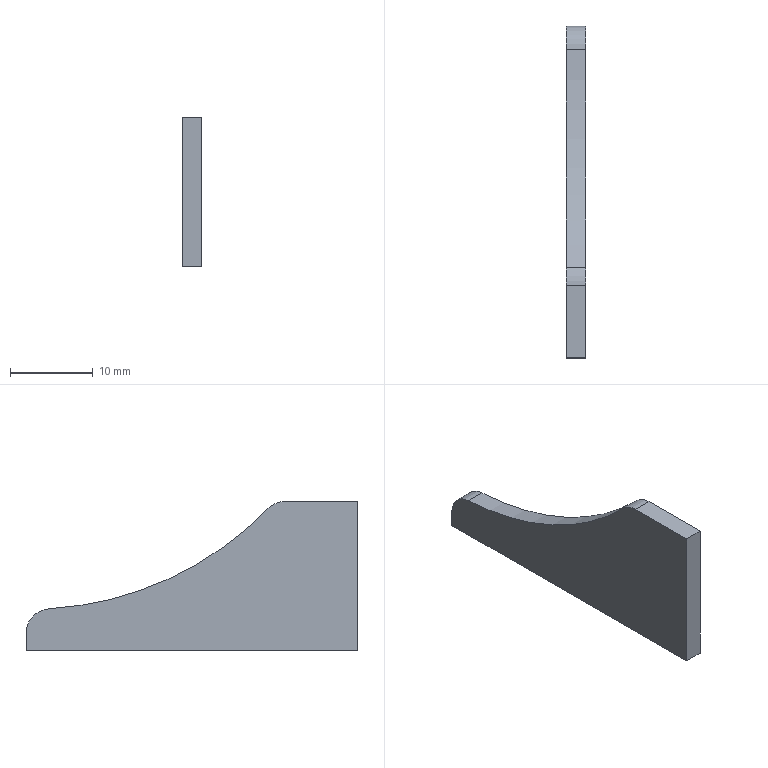Part | SolidWorks | features Fillet 1, FlatPattern 1, SMBaseFlange 1, SheetMetal 1 | 1 solid | 9 faces | box 2.3 x 40 x 18 mm | volume 1026 mm3 | plane 6 | cylinder 3 | commonest cylinder face diameters 6 x2 80 x1
STEP:
#1=CARTESIAN_POINT('',(0.,8.707,18.));
#2=VERTEX_POINT('',#1);
#3=CARTESIAN_POINT('',(0.,0.,18.));
#4=VERTEX_POINT('',#3);
#5=CARTESIAN_POINT('',(0.,10.,18.));
#6=DIRECTION('',(0.,-1.,0.));
#7=VECTOR('',#6,1000.);
#8=LINE('',#5,#7);
#9=EDGE_CURVE('',#2,#4,#8,.T.);
#10=ORIENTED_EDGE('',*,*,#9,.F.);
#11=CARTESIAN_POINT('',(-2.3,8.707,18.));
#12=VERTEX_POINT('',#11);
#13=CARTESIAN_POINT('',(-2.3,8.707,18.));
#14=DIRECTION('',(-1.,0.,0.));
#15=VECTOR('',#14,1000.);
#16=LINE('',#13,#15);
#17=EDGE_CURVE('',#2,#12,#16,.T.);
#18=ORIENTED_EDGE('',*,*,#17,.T.);
#19=CARTESIAN_POINT('',(-2.3,0.,18.));
#20=VERTEX_POINT('',#19);
#21=CARTESIAN_POINT('',(-2.3,10.,18.));
#22=DIRECTION('',(0.,-1.,0.));
#23=VECTOR('',#22,1000.);
#24=LINE('',#21,#23);
#25=EDGE_CURVE('',#12,#20,#24,.T.);
#26=ORIENTED_EDGE('',*,*,#25,.T.);
#27=CARTESIAN_POINT('',(-2.3,0.,18.));
#28=DIRECTION('',(1.,0.,0.));
#29=VECTOR('',#28,1000.);
#30=LINE('',#27,#29);
#31=EDGE_CURVE('',#20,#4,#30,.T.);
#32=ORIENTED_EDGE('',*,*,#31,.T.);
#33=EDGE_LOOP('',(#10,#18,#26,#32));
#34=FACE_OUTER_BOUND('',#33,.T.);
#35=CARTESIAN_POINT('',(-2.3,10.,18.));
#36=DIRECTION('',(0.,0.,1.));
#37=DIRECTION('',(1.,0.,0.));
#38=AXIS2_PLACEMENT_3D('',#35,#36,#37);
#39=PLANE('',#38);
#40=ADVANCED_FACE('',(#34),#39,.T.);
#41=CARTESIAN_POINT('',(-2.3,37.175,5.066));
#42=VERTEX_POINT('',#41);
#43=CARTESIAN_POINT('',(-2.3,10.856,17.093));
#44=VERTEX_POINT('',#43);
#45=CARTESIAN_POINT('',(-2.3,39.515,44.997));
#46=DIRECTION('',(-1.,0.,0.));
#47=DIRECTION('',(0.,0.,1.));
#48=AXIS2_PLACEMENT_3D('',#45,#46,#47);
#49=CIRCLE('',#48,40.);
#50=EDGE_CURVE('',#42,#44,#49,.T.);
#51=ORIENTED_EDGE('',*,*,#50,.T.);
#52=CARTESIAN_POINT('',(0.,10.856,17.093));
#53=VERTEX_POINT('',#52);
#54=CARTESIAN_POINT('',(-2.3,10.856,17.093));
#55=DIRECTION('',(1.,0.,0.));
#56=VECTOR('',#55,1000.);
#57=LINE('',#54,#56);
#58=EDGE_CURVE('',#44,#53,#57,.T.);
#59=ORIENTED_EDGE('',*,*,#58,.T.);
#60=CARTESIAN_POINT('',(0.,37.175,5.066));
#61=VERTEX_POINT('',#60);
#62=CARTESIAN_POINT('',(0.,39.515,44.997));
#63=DIRECTION('',(-1.,0.,0.));
#64=DIRECTION('',(0.,0.,1.));
#65=AXIS2_PLACEMENT_3D('',#62,#63,#64);
#66=CIRCLE('',#65,40.);
#67=EDGE_CURVE('',#61,#53,#66,.T.);
#68=ORIENTED_EDGE('',*,*,#67,.F.);
#69=CARTESIAN_POINT('',(-2.3,37.175,5.066));
#70=DIRECTION('',(-1.,0.,0.));
#71=VECTOR('',#70,1000.);
#72=LINE('',#69,#71);
#73=EDGE_CURVE('',#61,#42,#72,.T.);
#74=ORIENTED_EDGE('',*,*,#73,.T.);
#75=EDGE_LOOP('',(#51,#59,#68,#74));
#76=FACE_OUTER_BOUND('',#75,.T.);
#77=CARTESIAN_POINT('',(-2.3,39.515,44.997));
#78=DIRECTION('',(1.,0.,0.));
#79=DIRECTION('',(0.,0.,-1.));
#80=AXIS2_PLACEMENT_3D('',#77,#78,#79);
#81=CYLINDRICAL_SURFACE('',#80,40.);
#82=ADVANCED_FACE('',(#76),#81,.F.);
#83=CARTESIAN_POINT('',(-2.3,40.,0.));
#84=VERTEX_POINT('',#83);
#85=CARTESIAN_POINT('',(-2.3,40.,2.071));
#86=VERTEX_POINT('',#85);
#87=CARTESIAN_POINT('',(-2.3,40.,0.));
#88=DIRECTION('',(0.,0.,1.));
#89=VECTOR('',#88,1000.);
#90=LINE('',#87,#89);
#91=EDGE_CURVE('',#84,#86,#90,.T.);
#92=ORIENTED_EDGE('',*,*,#91,.T.);
#93=CARTESIAN_POINT('',(0.,40.,2.071));
#94=VERTEX_POINT('',#93);
#95=CARTESIAN_POINT('',(-2.3,40.,2.071));
#96=DIRECTION('',(1.,0.,0.));
#97=VECTOR('',#96,1000.);
#98=LINE('',#95,#97);
#99=EDGE_CURVE('',#86,#94,#98,.T.);
#100=ORIENTED_EDGE('',*,*,#99,.T.);
#101=CARTESIAN_POINT('',(0.,40.,0.));
#102=VERTEX_POINT('',#101);
#103=CARTESIAN_POINT('',(0.,40.,0.));
#104=DIRECTION('',(0.,0.,1.));
#105=VECTOR('',#104,1000.);
#106=LINE('',#103,#105);
#107=EDGE_CURVE('',#102,#94,#106,.T.);
#108=ORIENTED_EDGE('',*,*,#107,.F.);
#109=CARTESIAN_POINT('',(-2.3,40.,0.));
#110=DIRECTION('',(1.,0.,0.));
#111=VECTOR('',#110,1000.);
#112=LINE('',#109,#111);
#113=EDGE_CURVE('',#84,#102,#112,.T.);
#114=ORIENTED_EDGE('',*,*,#113,.F.);
#115=EDGE_LOOP('',(#92,#100,#108,#114));
#116=FACE_OUTER_BOUND('',#115,.T.);
#117=CARTESIAN_POINT('',(-2.3,40.,0.));
#118=DIRECTION('',(0.,1.,0.));
#119=DIRECTION('',(0.,0.,1.));
#120=AXIS2_PLACEMENT_3D('',#117,#118,#119);
#121=PLANE('',#120);
#122=ADVANCED_FACE('',(#116),#121,.T.);
#123=CARTESIAN_POINT('',(0.,0.,0.));
#124=VERTEX_POINT('',#123);
#125=CARTESIAN_POINT('',(0.,0.,0.));
#126=DIRECTION('',(0.,1.,0.));
#127=VECTOR('',#126,1000.);
#128=LINE('',#125,#127);
#129=EDGE_CURVE('',#124,#102,#128,.T.);
#130=ORIENTED_EDGE('',*,*,#129,.F.);
#131=CARTESIAN_POINT('',(-2.3,0.,0.));
#132=VERTEX_POINT('',#131);
#133=CARTESIAN_POINT('',(-2.3,0.,0.));
#134=DIRECTION('',(1.,0.,0.));
#135=VECTOR('',#134,1000.);
#136=LINE('',#133,#135);
#137=EDGE_CURVE('',#132,#124,#136,.T.);
#138=ORIENTED_EDGE('',*,*,#137,.F.);
#139=CARTESIAN_POINT('',(-2.3,0.,0.));
#140=DIRECTION('',(0.,1.,0.));
#141=VECTOR('',#140,1000.);
#142=LINE('',#139,#141);
#143=EDGE_CURVE('',#132,#84,#142,.T.);
#144=ORIENTED_EDGE('',*,*,#143,.T.);
#145=ORIENTED_EDGE('',*,*,#113,.T.);
#146=EDGE_LOOP('',(#130,#138,#144,#145));
#147=FACE_OUTER_BOUND('',#146,.T.);
#148=CARTESIAN_POINT('',(-2.3,0.,0.));
#149=DIRECTION('',(0.,0.,-1.));
#150=DIRECTION('',(-1.,0.,0.));
#151=AXIS2_PLACEMENT_3D('',#148,#149,#150);
#152=PLANE('',#151);
#153=ADVANCED_FACE('',(#147),#152,.T.);
#154=CARTESIAN_POINT('',(0.,0.,18.));
#155=DIRECTION('',(0.,0.,-1.));
#156=VECTOR('',#155,1000.);
#157=LINE('',#154,#156);
#158=EDGE_CURVE('',#4,#124,#157,.T.);
#159=ORIENTED_EDGE('',*,*,#158,.F.);
#160=ORIENTED_EDGE('',*,*,#31,.F.);
#161=CARTESIAN_POINT('',(-2.3,0.,18.));
#162=DIRECTION('',(0.,0.,-1.));
#163=VECTOR('',#162,1000.);
#164=LINE('',#161,#163);
#165=EDGE_CURVE('',#20,#132,#164,.T.);
#166=ORIENTED_EDGE('',*,*,#165,.T.);
#167=ORIENTED_EDGE('',*,*,#137,.T.);
#168=EDGE_LOOP('',(#159,#160,#166,#167));
#169=FACE_OUTER_BOUND('',#168,.T.);
#170=CARTESIAN_POINT('',(-2.3,0.,18.));
#171=DIRECTION('',(0.,-1.,0.));
#172=DIRECTION('',(0.,0.,-1.));
#173=AXIS2_PLACEMENT_3D('',#170,#171,#172);
#174=PLANE('',#173);
#175=ADVANCED_FACE('',(#169),#174,.T.);
#176=ORIENTED_EDGE('',*,*,#25,.F.);
#177=CARTESIAN_POINT('',(-2.3,8.707,15.));
#178=DIRECTION('',(-1.,0.,0.));
#179=DIRECTION('',(0.,0.,1.));
#180=AXIS2_PLACEMENT_3D('',#177,#178,#179);
#181=CIRCLE('',#180,3.);
#182=EDGE_CURVE('',#12,#44,#181,.T.);
#183=ORIENTED_EDGE('',*,*,#182,.T.);
#184=ORIENTED_EDGE('',*,*,#50,.F.);
#185=CARTESIAN_POINT('',(-2.3,37.,2.071));
#186=DIRECTION('',(-1.,0.,0.));
#187=DIRECTION('',(0.,0.,1.));
#188=AXIS2_PLACEMENT_3D('',#185,#186,#187);
#189=CIRCLE('',#188,3.);
#190=EDGE_CURVE('',#42,#86,#189,.T.);
#191=ORIENTED_EDGE('',*,*,#190,.T.);
#192=ORIENTED_EDGE('',*,*,#91,.F.);
#193=ORIENTED_EDGE('',*,*,#143,.F.);
#194=ORIENTED_EDGE('',*,*,#165,.F.);
#195=EDGE_LOOP('',(#176,#183,#184,#191,#192,#193,#194));
#196=FACE_OUTER_BOUND('',#195,.T.);
#197=CARTESIAN_POINT('',(-2.3,39.515,44.997));
#198=DIRECTION('',(-1.,0.,0.));
#199=DIRECTION('',(0.,0.,1.));
#200=AXIS2_PLACEMENT_3D('',#197,#198,#199);
#201=PLANE('',#200);
#202=ADVANCED_FACE('',(#196),#201,.T.);
#203=ORIENTED_EDGE('',*,*,#67,.T.);
#204=CARTESIAN_POINT('',(0.,8.707,15.));
#205=DIRECTION('',(1.,0.,0.));
#206=DIRECTION('',(0.,0.,1.));
#207=AXIS2_PLACEMENT_3D('',#204,#205,#206);
#208=CIRCLE('',#207,3.);
#209=EDGE_CURVE('',#53,#2,#208,.T.);
#210=ORIENTED_EDGE('',*,*,#209,.T.);
#211=ORIENTED_EDGE('',*,*,#9,.T.);
#212=ORIENTED_EDGE('',*,*,#158,.T.);
#213=ORIENTED_EDGE('',*,*,#129,.T.);
#214=ORIENTED_EDGE('',*,*,#107,.T.);
#215=CARTESIAN_POINT('',(0.,37.,2.071));
#216=DIRECTION('',(1.,0.,0.));
#217=DIRECTION('',(0.,0.,1.));
#218=AXIS2_PLACEMENT_3D('',#215,#216,#217);
#219=CIRCLE('',#218,3.);
#220=EDGE_CURVE('',#94,#61,#219,.T.);
#221=ORIENTED_EDGE('',*,*,#220,.T.);
#222=EDGE_LOOP('',(#203,#210,#211,#212,#213,#214,#221));
#223=FACE_OUTER_BOUND('',#222,.T.);
#224=CARTESIAN_POINT('',(0.,39.515,44.997));
#225=DIRECTION('',(-1.,0.,0.));
#226=DIRECTION('',(0.,0.,1.));
#227=AXIS2_PLACEMENT_3D('',#224,#225,#226);
#228=PLANE('',#227);
#229=ADVANCED_FACE('',(#223),#228,.F.);
#230=ORIENTED_EDGE('',*,*,#182,.F.);
#231=ORIENTED_EDGE('',*,*,#17,.F.);
#232=ORIENTED_EDGE('',*,*,#209,.F.);
#233=ORIENTED_EDGE('',*,*,#58,.F.);
#234=EDGE_LOOP('',(#230,#231,#232,#233));
#235=FACE_OUTER_BOUND('',#234,.T.);
#236=CARTESIAN_POINT('',(-2.3,8.707,15.));
#237=DIRECTION('',(1.,0.,0.));
#238=DIRECTION('',(0.,0.,-1.));
#239=AXIS2_PLACEMENT_3D('',#236,#237,#238);
#240=CYLINDRICAL_SURFACE('',#239,3.);
#241=ADVANCED_FACE('',(#235),#240,.T.);
#242=ORIENTED_EDGE('',*,*,#190,.F.);
#243=ORIENTED_EDGE('',*,*,#73,.F.);
#244=ORIENTED_EDGE('',*,*,#220,.F.);
#245=ORIENTED_EDGE('',*,*,#99,.F.);
#246=EDGE_LOOP('',(#242,#243,#244,#245));
#247=FACE_OUTER_BOUND('',#246,.T.);
#248=CARTESIAN_POINT('',(-2.3,37.,2.071));
#249=DIRECTION('',(1.,0.,0.));
#250=DIRECTION('',(0.,0.,-1.));
#251=AXIS2_PLACEMENT_3D('',#248,#249,#250);
#252=CYLINDRICAL_SURFACE('',#251,3.);
#253=ADVANCED_FACE('',(#247),#252,.T.);
#254=CLOSED_SHELL('',(#40,#82,#122,#153,#175,#202,#229,#241,#253));
#255=MANIFOLD_SOLID_BREP('',#254);
#256=CARTESIAN_POINT('',(0.,0.,0.));
#257=DIRECTION('',(0.,0.,1.));
#258=DIRECTION('',(1.,0.,0.));
#259=AXIS2_PLACEMENT_3D('',#256,#257,#258);
#260=(LENGTH_UNIT()NAMED_UNIT(*)SI_UNIT(.MILLI.,.METRE.));
#261=UNCERTAINTY_MEASURE_WITH_UNIT(LENGTH_MEASURE(0.00001),#260,'','');
#262=(NAMED_UNIT(*)PLANE_ANGLE_UNIT()SI_UNIT($,.RADIAN.));
#263=(NAMED_UNIT(*)SI_UNIT($,.STERADIAN.)SOLID_ANGLE_UNIT());
#264=(GEOMETRIC_REPRESENTATION_CONTEXT(3)GLOBAL_UNCERTAINTY_ASSIGNED_CONTEXT((#261))GLOBAL_UNIT_ASSIGNED_CONTEXT((#260,#262,#263))REPRESENTATION_CONTEXT('',''));
#265=ADVANCED_BREP_SHAPE_REPRESENTATION('',(#255,#259),#264);